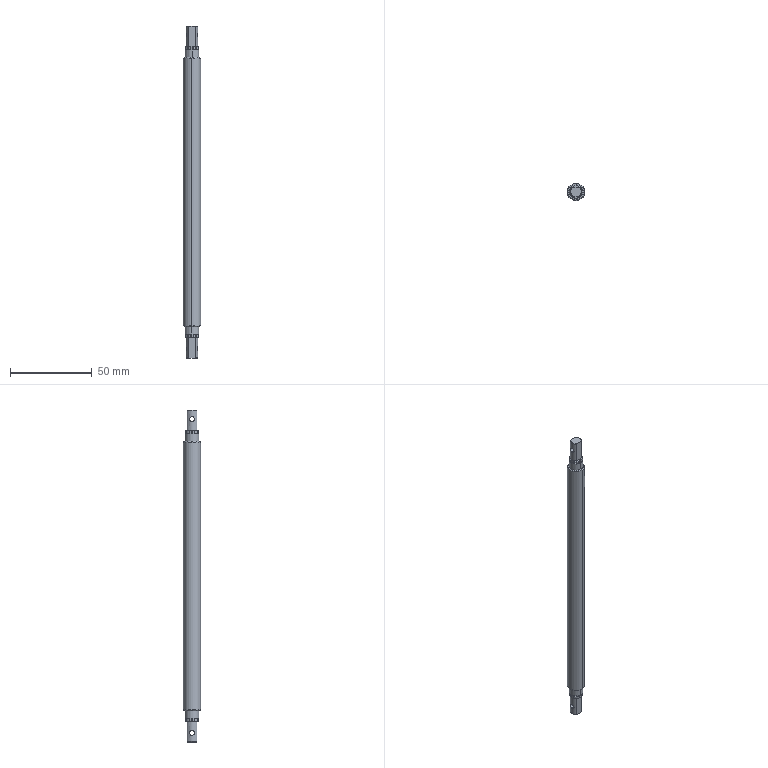Part | SolidWorks | features SplitBody 1 | 1 solid | 48 faces | box 10.5 x 10.5 x 203 mm | volume 15721 mm3 | cylinder 22 | plane 14 | cone 12 | commonest cylinder face diameters 7 x8 8.4 x8 2.94 x4 10.5 x2